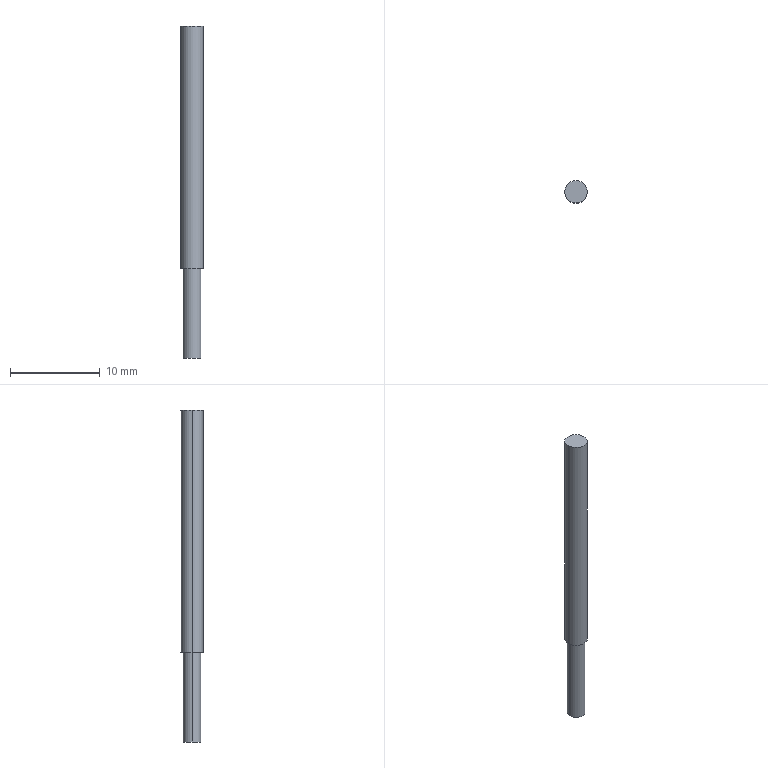Part | STEP file | D05 | 1 solid | 7 faces | box 2.5 x 2.5 x 37 mm | volume 163.952 mm3 | cylinder 4 | plane 3 | commonest cylinder face diameters 2 x2 2.5 x2
STEP:
#1=CARTESIAN_POINT('',(0.,0.,0.));
#2=DIRECTION('',(0.,0.,1.));
#3=DIRECTION('',(1.,0.,0.));
#4=AXIS2_PLACEMENT_3D('',#1,#2,#3);
#5=CARTESIAN_POINT('',(-1.,0.,-10.));
#6=VERTEX_POINT('',#5);
#7=CARTESIAN_POINT('',(1.,0.,-10.));
#8=VERTEX_POINT('',#7);
#9=CARTESIAN_POINT('',(0.,0.,-10.));
#10=DIRECTION('',(0.,0.,-1.));
#11=DIRECTION('',(-1.,0.,0.));
#12=AXIS2_PLACEMENT_3D('',#9,#10,#11);
#13=CIRCLE('',#12,1.);
#14=CARTESIAN_POINT('',(0.,0.,-10.));
#15=DIRECTION('',(0.,0.,1.));
#16=DIRECTION('',(1.,0.,0.));
#17=AXIS2_PLACEMENT_3D('',#14,#15,#16);
#18=CYLINDRICAL_SURFACE('',#17,1.);
#19=CARTESIAN_POINT('',(3.142,0.));
#20=DIRECTION('',(-1.,0.));
#21=VECTOR('',#20,1.);
#22=LINE('',#19,#21);
#23=(GEOMETRIC_REPRESENTATION_CONTEXT(2)PARAMETRIC_REPRESENTATION_CONTEXT()REPRESENTATION_CONTEXT('',''));
#24=DEFINITIONAL_REPRESENTATION('',(#22),#23);
#25=PCURVE('',#18,#24);
#26=CARTESIAN_POINT('',(0.,0.,-10.));
#27=DIRECTION('',(0.,0.,-1.));
#28=DIRECTION('',(-1.,0.,0.));
#29=AXIS2_PLACEMENT_3D('',#26,#27,#28);
#30=PLANE('',#29);
#31=CARTESIAN_POINT('',(0.,0.));
#32=DIRECTION('',(1.,0.));
#33=AXIS2_PLACEMENT_2D('',#31,#32);
#34=CIRCLE('',#33,1.);
#35=(GEOMETRIC_REPRESENTATION_CONTEXT(2)PARAMETRIC_REPRESENTATION_CONTEXT()REPRESENTATION_CONTEXT('',''));
#36=DEFINITIONAL_REPRESENTATION('',(#34),#35);
#37=PCURVE('',#30,#36);
#38=SURFACE_CURVE('',#13,(#25,#37),.PCURVE_S1.);
#39=EDGE_CURVE('',#6,#8,#38,.T.);
#40=ORIENTED_EDGE('',*,*,#39,.F.);
#41=CARTESIAN_POINT('',(-1.,0.,0.));
#42=VERTEX_POINT('',#41);
#43=CARTESIAN_POINT('',(-1.,0.,-10.));
#44=DIRECTION('',(0.,0.,1.));
#45=VECTOR('',#44,1.);
#46=LINE('',#43,#45);
#47=CARTESIAN_POINT('',(3.142,0.));
#48=DIRECTION('',(0.,1.));
#49=VECTOR('',#48,1.);
#50=LINE('',#47,#49);
#51=(GEOMETRIC_REPRESENTATION_CONTEXT(2)PARAMETRIC_REPRESENTATION_CONTEXT()REPRESENTATION_CONTEXT('',''));
#52=DEFINITIONAL_REPRESENTATION('',(#50),#51);
#53=PCURVE('',#18,#52);
#54=CARTESIAN_POINT('',(0.,0.,-10.));
#55=DIRECTION('',(0.,0.,1.));
#56=DIRECTION('',(1.,0.,0.));
#57=AXIS2_PLACEMENT_3D('',#54,#55,#56);
#58=CYLINDRICAL_SURFACE('',#57,1.);
#59=CARTESIAN_POINT('',(3.142,0.));
#60=DIRECTION('',(0.,1.));
#61=VECTOR('',#60,1.);
#62=LINE('',#59,#61);
#63=(GEOMETRIC_REPRESENTATION_CONTEXT(2)PARAMETRIC_REPRESENTATION_CONTEXT()REPRESENTATION_CONTEXT('',''));
#64=DEFINITIONAL_REPRESENTATION('',(#62),#63);
#65=PCURVE('',#58,#64);
#66=SURFACE_CURVE('',#46,(#53,#65),.PCURVE_S1.);
#67=EDGE_CURVE('',#6,#42,#66,.T.);
#68=ORIENTED_EDGE('',*,*,#67,.T.);
#69=CARTESIAN_POINT('',(1.,0.,0.));
#70=VERTEX_POINT('',#69);
#71=CARTESIAN_POINT('',(0.,0.,0.));
#72=DIRECTION('',(0.,0.,-1.));
#73=DIRECTION('',(1.,0.,0.));
#74=AXIS2_PLACEMENT_3D('',#71,#72,#73);
#75=CIRCLE('',#74,1.);
#76=CARTESIAN_POINT('',(6.283,10.));
#77=DIRECTION('',(-1.,0.));
#78=VECTOR('',#77,1.);
#79=LINE('',#76,#78);
#80=(GEOMETRIC_REPRESENTATION_CONTEXT(2)PARAMETRIC_REPRESENTATION_CONTEXT()REPRESENTATION_CONTEXT('',''));
#81=DEFINITIONAL_REPRESENTATION('',(#79),#80);
#82=PCURVE('',#18,#81);
#83=CARTESIAN_POINT('',(0.,0.,0.));
#84=DIRECTION('',(0.,0.,1.));
#85=DIRECTION('',(1.,0.,0.));
#86=AXIS2_PLACEMENT_3D('',#83,#84,#85);
#87=PLANE('',#86);
#88=CARTESIAN_POINT('',(1.,0.));
#89=CARTESIAN_POINT('',(1.,-1.732));
#90=CARTESIAN_POINT('',(-0.5,-0.866));
#91=CARTESIAN_POINT('',(-2.,0.));
#92=CARTESIAN_POINT('',(-0.5,0.866));
#93=CARTESIAN_POINT('',(1.,1.732));
#94=CARTESIAN_POINT('',(1.,0.));
#95=(BOUNDED_CURVE()B_SPLINE_CURVE(2,(#88,#89,#90,#91,#92,#93,#94),.UNSPECIFIED.,.T.,.F.)B_SPLINE_CURVE_WITH_KNOTS((1,2,2,2,2,1),(-2.094,0.,2.094,4.189,6.283,8.378),.UNSPECIFIED.)CURVE()GEOMETRIC_REPRESENTATION_ITEM()RATIONAL_B_SPLINE_CURVE((1.,0.5,1.,0.5,1.,0.5,1.))REPRESENTATION_ITEM(''));
#96=(GEOMETRIC_REPRESENTATION_CONTEXT(2)PARAMETRIC_REPRESENTATION_CONTEXT()REPRESENTATION_CONTEXT('',''));
#97=DEFINITIONAL_REPRESENTATION('',(#95),#96);
#98=PCURVE('',#87,#97);
#99=SURFACE_CURVE('',#75,(#82,#98),.PCURVE_S1.);
#100=EDGE_CURVE('',#42,#70,#99,.T.);
#101=ORIENTED_EDGE('',*,*,#100,.T.);
#102=CARTESIAN_POINT('',(1.,0.,-10.));
#103=DIRECTION('',(0.,0.,1.));
#104=VECTOR('',#103,1.);
#105=LINE('',#102,#104);
#106=CARTESIAN_POINT('',(0.,0.));
#107=DIRECTION('',(0.,1.));
#108=VECTOR('',#107,1.);
#109=LINE('',#106,#108);
#110=(GEOMETRIC_REPRESENTATION_CONTEXT(2)PARAMETRIC_REPRESENTATION_CONTEXT()REPRESENTATION_CONTEXT('',''));
#111=DEFINITIONAL_REPRESENTATION('',(#109),#110);
#112=PCURVE('',#18,#111);
#113=CARTESIAN_POINT('',(6.283,0.));
#114=DIRECTION('',(0.,1.));
#115=VECTOR('',#114,1.);
#116=LINE('',#113,#115);
#117=(GEOMETRIC_REPRESENTATION_CONTEXT(2)PARAMETRIC_REPRESENTATION_CONTEXT()REPRESENTATION_CONTEXT('',''));
#118=DEFINITIONAL_REPRESENTATION('',(#116),#117);
#119=PCURVE('',#58,#118);
#120=SURFACE_CURVE('',#105,(#112,#119),.PCURVE_S1.);
#121=EDGE_CURVE('',#8,#70,#120,.T.);
#122=ORIENTED_EDGE('',*,*,#121,.F.);
#123=EDGE_LOOP('',(#40,#68,#101,#122));
#124=FACE_BOUND('',#123,.T.);
#125=ADVANCED_FACE('',(#124),#18,.T.);
#126=CARTESIAN_POINT('',(1.25,0.,27.));
#127=VERTEX_POINT('',#126);
#128=CARTESIAN_POINT('',(-1.25,0.,27.));
#129=VERTEX_POINT('',#128);
#130=CARTESIAN_POINT('',(0.,0.,27.));
#131=DIRECTION('',(0.,0.,1.));
#132=DIRECTION('',(1.,0.,0.));
#133=AXIS2_PLACEMENT_3D('',#130,#131,#132);
#134=CIRCLE('',#133,1.25);
#135=CARTESIAN_POINT('',(0.,0.,27.));
#136=DIRECTION('',(0.,0.,-1.));
#137=DIRECTION('',(-1.,0.,0.));
#138=AXIS2_PLACEMENT_3D('',#135,#136,#137);
#139=CYLINDRICAL_SURFACE('',#138,1.25);
#140=CARTESIAN_POINT('',(3.142,0.));
#141=DIRECTION('',(-1.,0.));
#142=VECTOR('',#141,1.);
#143=LINE('',#140,#142);
#144=(GEOMETRIC_REPRESENTATION_CONTEXT(2)PARAMETRIC_REPRESENTATION_CONTEXT()REPRESENTATION_CONTEXT('',''));
#145=DEFINITIONAL_REPRESENTATION('',(#143),#144);
#146=PCURVE('',#139,#145);
#147=CARTESIAN_POINT('',(0.,0.,27.));
#148=DIRECTION('',(0.,0.,1.));
#149=DIRECTION('',(1.,0.,0.));
#150=AXIS2_PLACEMENT_3D('',#147,#148,#149);
#151=PLANE('',#150);
#152=CARTESIAN_POINT('',(0.,0.));
#153=DIRECTION('',(1.,0.));
#154=AXIS2_PLACEMENT_2D('',#152,#153);
#155=CIRCLE('',#154,1.25);
#156=(GEOMETRIC_REPRESENTATION_CONTEXT(2)PARAMETRIC_REPRESENTATION_CONTEXT()REPRESENTATION_CONTEXT('',''));
#157=DEFINITIONAL_REPRESENTATION('',(#155),#156);
#158=PCURVE('',#151,#157);
#159=SURFACE_CURVE('',#134,(#146,#158),.PCURVE_S1.);
#160=EDGE_CURVE('',#127,#129,#159,.T.);
#161=ORIENTED_EDGE('',*,*,#160,.F.);
#162=CARTESIAN_POINT('',(1.25,0.,0.));
#163=VERTEX_POINT('',#162);
#164=CARTESIAN_POINT('',(1.25,0.,27.));
#165=DIRECTION('',(0.,0.,-1.));
#166=VECTOR('',#165,1.);
#167=LINE('',#164,#166);
#168=CARTESIAN_POINT('',(3.142,0.));
#169=DIRECTION('',(0.,1.));
#170=VECTOR('',#169,1.);
#171=LINE('',#168,#170);
#172=(GEOMETRIC_REPRESENTATION_CONTEXT(2)PARAMETRIC_REPRESENTATION_CONTEXT()REPRESENTATION_CONTEXT('',''));
#173=DEFINITIONAL_REPRESENTATION('',(#171),#172);
#174=PCURVE('',#139,#173);
#175=CARTESIAN_POINT('',(0.,0.,27.));
#176=DIRECTION('',(0.,0.,-1.));
#177=DIRECTION('',(-1.,0.,0.));
#178=AXIS2_PLACEMENT_3D('',#175,#176,#177);
#179=CYLINDRICAL_SURFACE('',#178,1.25);
#180=CARTESIAN_POINT('',(3.142,0.));
#181=DIRECTION('',(0.,1.));
#182=VECTOR('',#181,1.);
#183=LINE('',#180,#182);
#184=(GEOMETRIC_REPRESENTATION_CONTEXT(2)PARAMETRIC_REPRESENTATION_CONTEXT()REPRESENTATION_CONTEXT('',''));
#185=DEFINITIONAL_REPRESENTATION('',(#183),#184);
#186=PCURVE('',#179,#185);
#187=SURFACE_CURVE('',#167,(#174,#186),.PCURVE_S1.);
#188=EDGE_CURVE('',#127,#163,#187,.T.);
#189=ORIENTED_EDGE('',*,*,#188,.T.);
#190=CARTESIAN_POINT('',(-1.25,0.,0.));
#191=VERTEX_POINT('',#190);
#192=CARTESIAN_POINT('',(0.,0.,0.));
#193=DIRECTION('',(0.,0.,1.));
#194=DIRECTION('',(1.,0.,0.));
#195=AXIS2_PLACEMENT_3D('',#192,#193,#194);
#196=CIRCLE('',#195,1.25);
#197=CARTESIAN_POINT('',(3.142,27.));
#198=DIRECTION('',(-1.,0.));
#199=VECTOR('',#198,1.);
#200=LINE('',#197,#199);
#201=(GEOMETRIC_REPRESENTATION_CONTEXT(2)PARAMETRIC_REPRESENTATION_CONTEXT()REPRESENTATION_CONTEXT('',''));
#202=DEFINITIONAL_REPRESENTATION('',(#200),#201);
#203=PCURVE('',#139,#202);
#204=CARTESIAN_POINT('',(0.,0.));
#205=DIRECTION('',(1.,0.));
#206=AXIS2_PLACEMENT_2D('',#204,#205);
#207=CIRCLE('',#206,1.25);
#208=(GEOMETRIC_REPRESENTATION_CONTEXT(2)PARAMETRIC_REPRESENTATION_CONTEXT()REPRESENTATION_CONTEXT('',''));
#209=DEFINITIONAL_REPRESENTATION('',(#207),#208);
#210=PCURVE('',#87,#209);
#211=SURFACE_CURVE('',#196,(#203,#210),.PCURVE_S1.);
#212=EDGE_CURVE('',#163,#191,#211,.T.);
#213=ORIENTED_EDGE('',*,*,#212,.T.);
#214=CARTESIAN_POINT('',(-1.25,0.,27.));
#215=DIRECTION('',(0.,0.,-1.));
#216=VECTOR('',#215,1.);
#217=LINE('',#214,#216);
#218=CARTESIAN_POINT('',(0.,0.));
#219=DIRECTION('',(0.,1.));
#220=VECTOR('',#219,1.);
#221=LINE('',#218,#220);
#222=(GEOMETRIC_REPRESENTATION_CONTEXT(2)PARAMETRIC_REPRESENTATION_CONTEXT()REPRESENTATION_CONTEXT('',''));
#223=DEFINITIONAL_REPRESENTATION('',(#221),#222);
#224=PCURVE('',#139,#223);
#225=CARTESIAN_POINT('',(6.283,0.));
#226=DIRECTION('',(0.,1.));
#227=VECTOR('',#226,1.);
#228=LINE('',#225,#227);
#229=(GEOMETRIC_REPRESENTATION_CONTEXT(2)PARAMETRIC_REPRESENTATION_CONTEXT()REPRESENTATION_CONTEXT('',''));
#230=DEFINITIONAL_REPRESENTATION('',(#228),#229);
#231=PCURVE('',#179,#230);
#232=SURFACE_CURVE('',#217,(#224,#231),.PCURVE_S1.);
#233=EDGE_CURVE('',#129,#191,#232,.T.);
#234=ORIENTED_EDGE('',*,*,#233,.F.);
#235=EDGE_LOOP('',(#161,#189,#213,#234));
#236=FACE_BOUND('',#235,.T.);
#237=ADVANCED_FACE('',(#236),#139,.T.);
#238=CARTESIAN_POINT('',(0.,0.,0.));
#239=DIRECTION('',(0.,0.,1.));
#240=DIRECTION('',(1.,0.,0.));
#241=AXIS2_PLACEMENT_3D('',#238,#239,#240);
#242=CIRCLE('',#241,1.25);
#243=CARTESIAN_POINT('',(0.,0.));
#244=DIRECTION('',(1.,0.));
#245=AXIS2_PLACEMENT_2D('',#243,#244);
#246=CIRCLE('',#245,1.25);
#247=(GEOMETRIC_REPRESENTATION_CONTEXT(2)PARAMETRIC_REPRESENTATION_CONTEXT()REPRESENTATION_CONTEXT('',''));
#248=DEFINITIONAL_REPRESENTATION('',(#246),#247);
#249=PCURVE('',#87,#248);
#250=CARTESIAN_POINT('',(9.425,27.));
#251=DIRECTION('',(-1.,0.));
#252=VECTOR('',#251,1.);
#253=LINE('',#250,#252);
#254=(GEOMETRIC_REPRESENTATION_CONTEXT(2)PARAMETRIC_REPRESENTATION_CONTEXT()REPRESENTATION_CONTEXT('',''));
#255=DEFINITIONAL_REPRESENTATION('',(#253),#254);
#256=PCURVE('',#179,#255);
#257=SURFACE_CURVE('',#242,(#249,#256),.PCURVE_S1.);
#258=EDGE_CURVE('',#191,#163,#257,.T.);
#259=ORIENTED_EDGE('',*,*,#258,.F.);
#260=ORIENTED_EDGE('',*,*,#212,.F.);
#261=EDGE_LOOP('',(#259,#260));
#262=FACE_BOUND('',#261,.T.);
#263=CARTESIAN_POINT('',(0.,0.,0.));
#264=DIRECTION('',(0.,0.,-1.));
#265=DIRECTION('',(1.,0.,0.));
#266=AXIS2_PLACEMENT_3D('',#263,#264,#265);
#267=CIRCLE('',#266,1.);
#268=CARTESIAN_POINT('',(1.,0.));
#269=CARTESIAN_POINT('',(1.,-1.732));
#270=CARTESIAN_POINT('',(-0.5,-0.866));
#271=CARTESIAN_POINT('',(-2.,0.));
#272=CARTESIAN_POINT('',(-0.5,0.866));
#273=CARTESIAN_POINT('',(1.,1.732));
#274=CARTESIAN_POINT('',(1.,0.));
#275=(BOUNDED_CURVE()B_SPLINE_CURVE(2,(#268,#269,#270,#271,#272,#273,#274),.UNSPECIFIED.,.T.,.F.)B_SPLINE_CURVE_WITH_KNOTS((1,2,2,2,2,1),(-2.094,0.,2.094,4.189,6.283,8.378),.UNSPECIFIED.)CURVE()GEOMETRIC_REPRESENTATION_ITEM()RATIONAL_B_SPLINE_CURVE((1.,0.5,1.,0.5,1.,0.5,1.))REPRESENTATION_ITEM(''));
#276=(GEOMETRIC_REPRESENTATION_CONTEXT(2)PARAMETRIC_REPRESENTATION_CONTEXT()REPRESENTATION_CONTEXT('',''));
#277=DEFINITIONAL_REPRESENTATION('',(#275),#276);
#278=PCURVE('',#87,#277);
#279=CARTESIAN_POINT('',(6.283,10.));
#280=DIRECTION('',(-1.,0.));
#281=VECTOR('',#280,1.);
#282=LINE('',#279,#281);
#283=(GEOMETRIC_REPRESENTATION_CONTEXT(2)PARAMETRIC_REPRESENTATION_CONTEXT()REPRESENTATION_CONTEXT('',''));
#284=DEFINITIONAL_REPRESENTATION('',(#282),#283);
#285=PCURVE('',#58,#284);
#286=SURFACE_CURVE('',#267,(#278,#285),.PCURVE_S1.);
#287=EDGE_CURVE('',#70,#42,#286,.T.);
#288=ORIENTED_EDGE('',*,*,#287,.F.);
#289=ORIENTED_EDGE('',*,*,#100,.F.);
#290=EDGE_LOOP('',(#288,#289));
#291=FACE_BOUND('',#290,.T.);
#292=ADVANCED_FACE('',(#262,#291),#87,.F.);
#293=ORIENTED_EDGE('',*,*,#188,.F.);
#294=CARTESIAN_POINT('',(0.,0.,27.));
#295=DIRECTION('',(0.,0.,1.));
#296=DIRECTION('',(1.,0.,0.));
#297=AXIS2_PLACEMENT_3D('',#294,#295,#296);
#298=CIRCLE('',#297,1.25);
#299=CARTESIAN_POINT('',(9.425,0.));
#300=DIRECTION('',(-1.,0.));
#301=VECTOR('',#300,1.);
#302=LINE('',#299,#301);
#303=(GEOMETRIC_REPRESENTATION_CONTEXT(2)PARAMETRIC_REPRESENTATION_CONTEXT()REPRESENTATION_CONTEXT('',''));
#304=DEFINITIONAL_REPRESENTATION('',(#302),#303);
#305=PCURVE('',#179,#304);
#306=CARTESIAN_POINT('',(0.,0.));
#307=DIRECTION('',(1.,0.));
#308=AXIS2_PLACEMENT_2D('',#306,#307);
#309=CIRCLE('',#308,1.25);
#310=(GEOMETRIC_REPRESENTATION_CONTEXT(2)PARAMETRIC_REPRESENTATION_CONTEXT()REPRESENTATION_CONTEXT('',''));
#311=DEFINITIONAL_REPRESENTATION('',(#309),#310);
#312=PCURVE('',#151,#311);
#313=SURFACE_CURVE('',#298,(#305,#312),.PCURVE_S1.);
#314=EDGE_CURVE('',#129,#127,#313,.T.);
#315=ORIENTED_EDGE('',*,*,#314,.F.);
#316=ORIENTED_EDGE('',*,*,#233,.T.);
#317=ORIENTED_EDGE('',*,*,#258,.T.);
#318=EDGE_LOOP('',(#293,#315,#316,#317));
#319=FACE_BOUND('',#318,.T.);
#320=ADVANCED_FACE('',(#319),#179,.T.);
#321=ORIENTED_EDGE('',*,*,#314,.T.);
#322=ORIENTED_EDGE('',*,*,#160,.T.);
#323=EDGE_LOOP('',(#321,#322));
#324=FACE_BOUND('',#323,.T.);
#325=ADVANCED_FACE('',(#324),#151,.T.);
#326=ORIENTED_EDGE('',*,*,#67,.F.);
#327=CARTESIAN_POINT('',(0.,0.,-10.));
#328=DIRECTION('',(0.,0.,-1.));
#329=DIRECTION('',(-1.,0.,0.));
#330=AXIS2_PLACEMENT_3D('',#327,#328,#329);
#331=CIRCLE('',#330,1.);
#332=CARTESIAN_POINT('',(9.425,0.));
#333=DIRECTION('',(-1.,0.));
#334=VECTOR('',#333,1.);
#335=LINE('',#332,#334);
#336=(GEOMETRIC_REPRESENTATION_CONTEXT(2)PARAMETRIC_REPRESENTATION_CONTEXT()REPRESENTATION_CONTEXT('',''));
#337=DEFINITIONAL_REPRESENTATION('',(#335),#336);
#338=PCURVE('',#58,#337);
#339=CARTESIAN_POINT('',(0.,0.));
#340=DIRECTION('',(1.,0.));
#341=AXIS2_PLACEMENT_2D('',#339,#340);
#342=CIRCLE('',#341,1.);
#343=(GEOMETRIC_REPRESENTATION_CONTEXT(2)PARAMETRIC_REPRESENTATION_CONTEXT()REPRESENTATION_CONTEXT('',''));
#344=DEFINITIONAL_REPRESENTATION('',(#342),#343);
#345=PCURVE('',#30,#344);
#346=SURFACE_CURVE('',#331,(#338,#345),.PCURVE_S1.);
#347=EDGE_CURVE('',#8,#6,#346,.T.);
#348=ORIENTED_EDGE('',*,*,#347,.F.);
#349=ORIENTED_EDGE('',*,*,#121,.T.);
#350=ORIENTED_EDGE('',*,*,#287,.T.);
#351=EDGE_LOOP('',(#326,#348,#349,#350));
#352=FACE_BOUND('',#351,.T.);
#353=ADVANCED_FACE('',(#352),#58,.T.);
#354=ORIENTED_EDGE('',*,*,#347,.T.);
#355=ORIENTED_EDGE('',*,*,#39,.T.);
#356=EDGE_LOOP('',(#354,#355));
#357=FACE_BOUND('',#356,.T.);
#358=ADVANCED_FACE('',(#357),#30,.T.);
#359=CLOSED_SHELL('',(#125,#237,#292,#320,#325,#353,#358));
#360=MANIFOLD_SOLID_BREP('',#359);
#361=(LENGTH_UNIT()NAMED_UNIT(*)SI_UNIT(.MILLI.,.METRE.));
#362=UNCERTAINTY_MEASURE_WITH_UNIT(LENGTH_MEASURE(0.0000001),#361,'','');
#363=(NAMED_UNIT(*)PLANE_ANGLE_UNIT()SI_UNIT($,.RADIAN.));
#364=(NAMED_UNIT(*)SI_UNIT($,.STERADIAN.)SOLID_ANGLE_UNIT());
#365=(GEOMETRIC_REPRESENTATION_CONTEXT(3)GLOBAL_UNCERTAINTY_ASSIGNED_CONTEXT((#362))GLOBAL_UNIT_ASSIGNED_CONTEXT((#361,#363,#364))REPRESENTATION_CONTEXT('',''));
#366=ADVANCED_BREP_SHAPE_REPRESENTATION('',(#4,#360),#365);